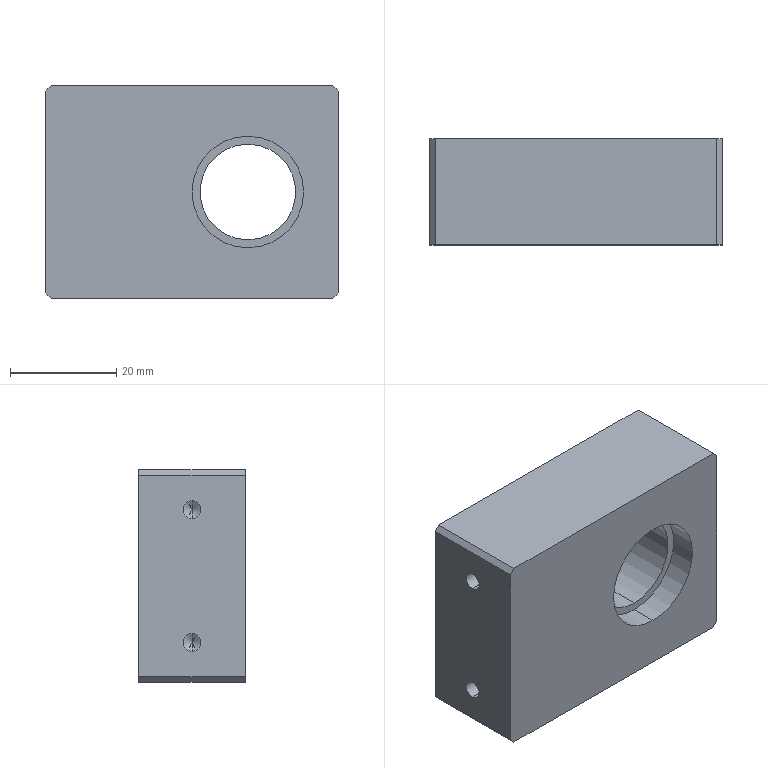Part | STEP file | PN_0036 | 1 solid | 26 faces | box 55 x 20 x 40 mm | volume 37681 mm3 | plane 12 | cylinder 10 | cone 4 | commonest cylinder face diameters 3.3 x4 21 x4 18 x2